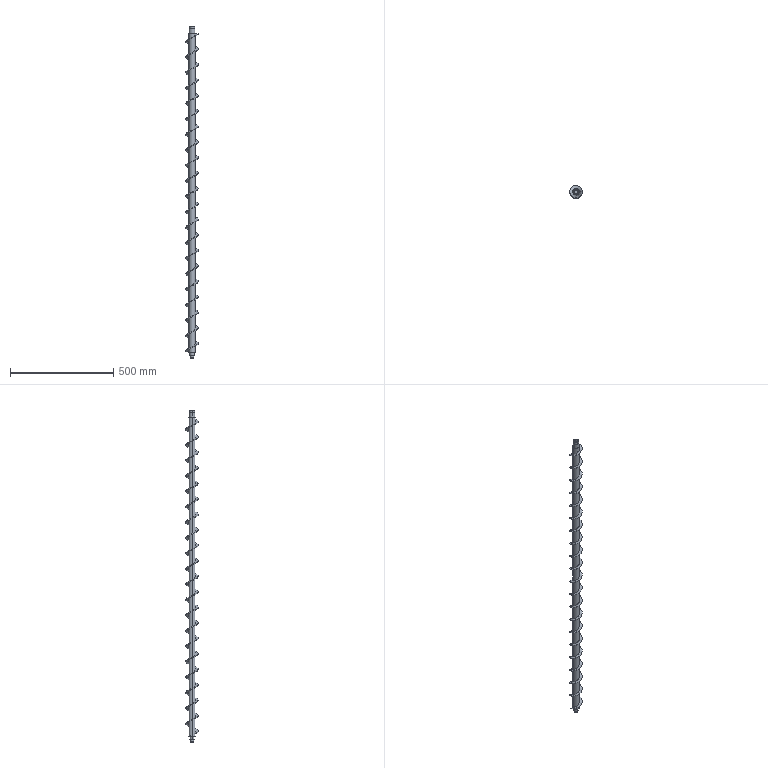Part | SolidWorks | features MoveFace 7, ICE 2, BaseBody 1, Helix 1, Sweep 1 | 2 solids | 34 faces | box 60 x 60 x 1608 mm | volume 669681 mm3 | cylinder 15 | plane 13 | spline 4 | cone 2 | commonest cylinder face diameters 25 x4 16 x3 17 x2 20 x2 28 x2 32 x2